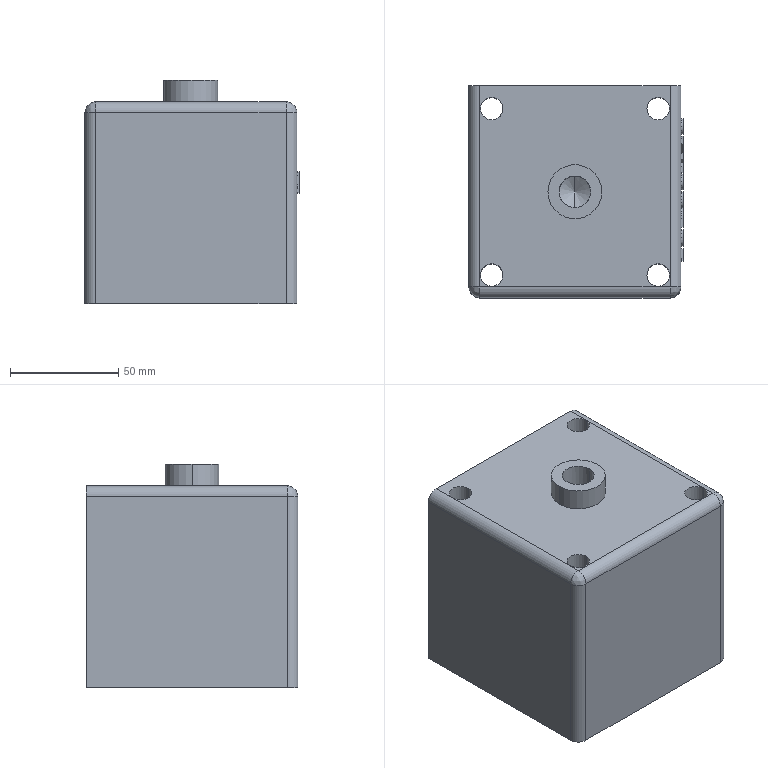Part | STEP file | JSR80X40 | 1 solid | 244 faces | box 99 x 98 x 103.5 mm | volume 861667 mm3 | spline 151 | plane 71 | cylinder 20 | cone 2 | commonest cylinder face diameters 10.441 x8 10 x5 14.676 x2 25 x2 16.727 x1 17.172 x1